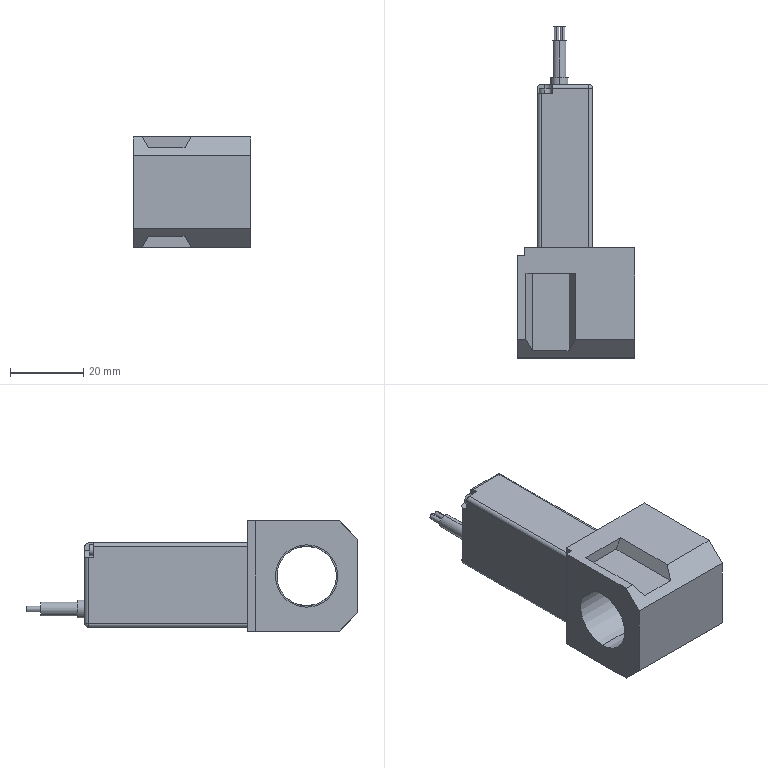Part | STEP file | IS1000E-3003-X202_IS1000E3035GA Body_30 | 1 solid | 64 faces | box 32 x 90.5 x 30 mm | volume 34770 mm3 | plane 36 | cylinder 24 | cone 2 | sphere 2 | commonest cylinder face diameters 2 x8 1.5 x4 3 x4 3.8 x2 4 x2 4.8 x2